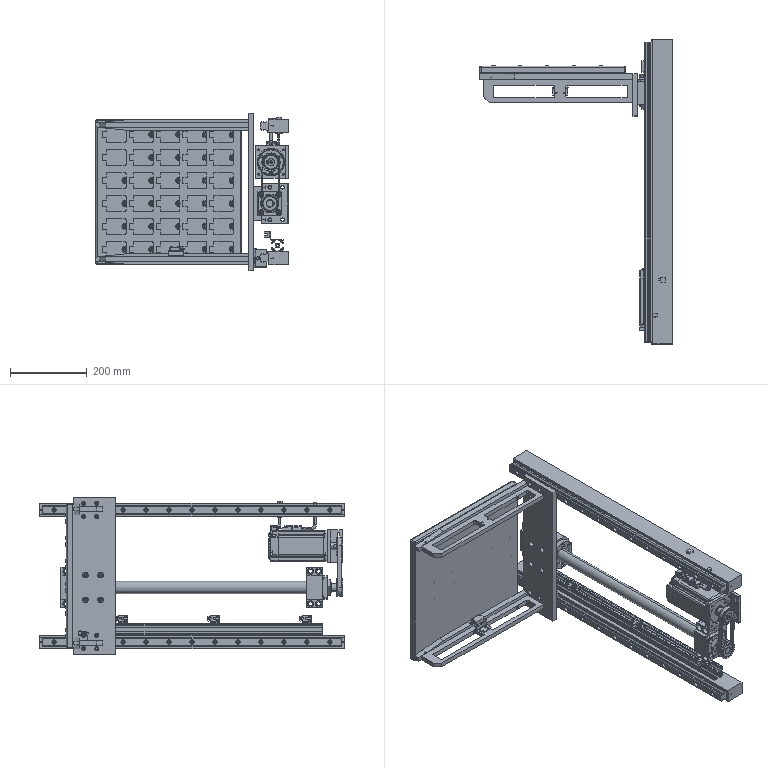Part | SolidWorks | features ReferencePattern 35, LocalLPattern 3, AEMSimFeature 1, CompositeCurve 1 | 113 solids | 48147 faces | volume 9390666 mm3 | cylinder 20357 | spline 14895 | plane 8030 | torus 4464 | cone 393 | sphere 8 | commonest cylinder face diameters 0.6 x14139 2 x835 1 x665 6 x520 11 x392 6.5 x352